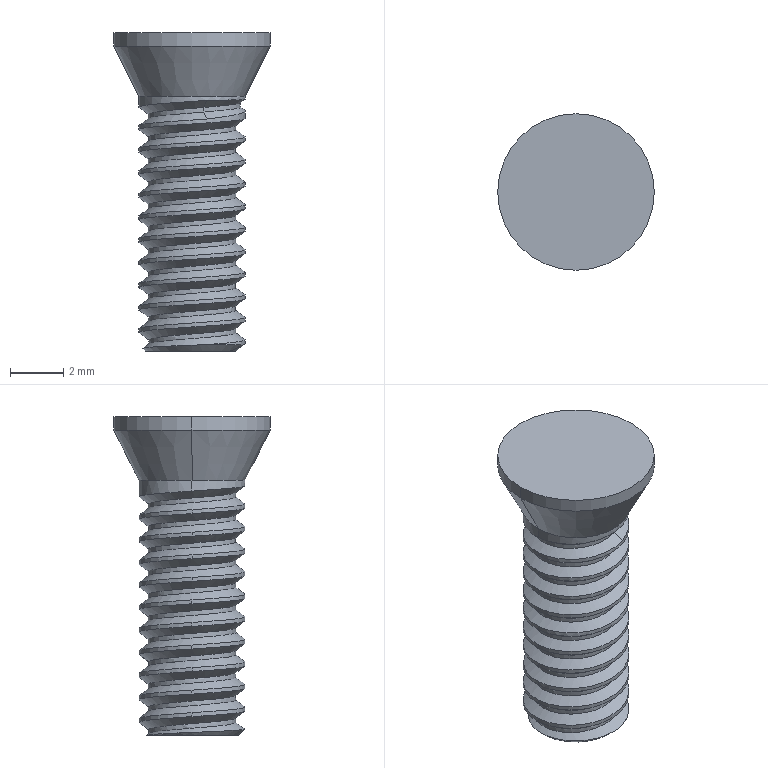Part | NX | features BREP 1 | 1 solid | 43 faces | volume 151.707 mm3 | cylinder 25 | spline 12 | cone 3 | plane 3 | commonest cylinder face diameters 4 x23 5.9 x2